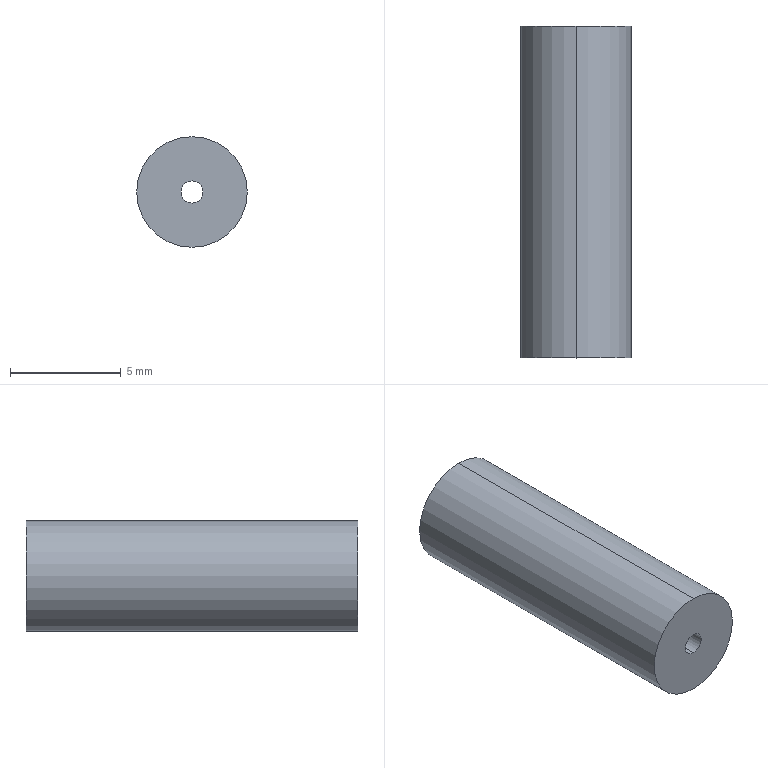Part | SolidWorks | features Extrusion 1, ICE 1 | 1 solid | 9 faces | box 5 x 15 x 5 mm | volume 201.062 mm3 | cylinder 6 | plane 3 | commonest cylinder face diameters 1 x2 3 x2 5 x2
STEP:
#1=CARTESIAN_POINT('',(0.,2.,0.5));
#2=VERTEX_POINT('',#1);
#3=CARTESIAN_POINT('',(0.,2.,-0.5));
#4=VERTEX_POINT('',#3);
#5=CARTESIAN_POINT('',(0.,2.,0.));
#6=DIRECTION('',(0.,-1.,0.));
#7=DIRECTION('',(0.,0.,-1.));
#8=AXIS2_PLACEMENT_3D('',#5,#6,#7);
#9=CIRCLE('',#8,0.5);
#10=EDGE_CURVE('',#2,#4,#9,.T.);
#11=ORIENTED_EDGE('',*,*,#10,.F.);
#12=CARTESIAN_POINT('',(0.,0.,0.5));
#13=VERTEX_POINT('',#12);
#14=CARTESIAN_POINT('',(0.,2.,0.5));
#15=DIRECTION('',(0.,-1.,0.));
#16=VECTOR('',#15,1000.);
#17=LINE('',#14,#16);
#18=EDGE_CURVE('',#2,#13,#17,.T.);
#19=ORIENTED_EDGE('',*,*,#18,.T.);
#20=CARTESIAN_POINT('',(0.,0.,-0.5));
#21=VERTEX_POINT('',#20);
#22=CARTESIAN_POINT('',(0.,0.,0.));
#23=DIRECTION('',(0.,-1.,0.));
#24=DIRECTION('',(0.,0.,-1.));
#25=AXIS2_PLACEMENT_3D('',#22,#23,#24);
#26=CIRCLE('',#25,0.5);
#27=EDGE_CURVE('',#13,#21,#26,.T.);
#28=ORIENTED_EDGE('',*,*,#27,.T.);
#29=CARTESIAN_POINT('',(0.,2.,-0.5));
#30=DIRECTION('',(0.,-1.,0.));
#31=VECTOR('',#30,1000.);
#32=LINE('',#29,#31);
#33=EDGE_CURVE('',#4,#21,#32,.T.);
#34=ORIENTED_EDGE('',*,*,#33,.F.);
#35=EDGE_LOOP('',(#11,#19,#28,#34));
#36=FACE_OUTER_BOUND('',#35,.T.);
#37=CARTESIAN_POINT('',(0.,2.,0.));
#38=DIRECTION('',(0.,-1.,0.));
#39=DIRECTION('',(0.,0.,-1.));
#40=AXIS2_PLACEMENT_3D('',#37,#38,#39);
#41=CYLINDRICAL_SURFACE('',#40,0.5);
#42=ADVANCED_FACE('',(#36),#41,.F.);
#43=CARTESIAN_POINT('',(0.,15.,2.5));
#44=VERTEX_POINT('',#43);
#45=CARTESIAN_POINT('',(0.,15.,-2.5));
#46=VERTEX_POINT('',#45);
#47=CARTESIAN_POINT('',(0.,15.,0.));
#48=DIRECTION('',(0.,1.,0.));
#49=DIRECTION('',(0.,0.,1.));
#50=AXIS2_PLACEMENT_3D('',#47,#48,#49);
#51=CIRCLE('',#50,2.5);
#52=EDGE_CURVE('',#44,#46,#51,.T.);
#53=ORIENTED_EDGE('',*,*,#52,.F.);
#54=CARTESIAN_POINT('',(0.,0.,2.5));
#55=VERTEX_POINT('',#54);
#56=CARTESIAN_POINT('',(0.,15.,2.5));
#57=DIRECTION('',(0.,-1.,0.));
#58=VECTOR('',#57,1000.);
#59=LINE('',#56,#58);
#60=EDGE_CURVE('',#44,#55,#59,.T.);
#61=ORIENTED_EDGE('',*,*,#60,.T.);
#62=CARTESIAN_POINT('',(0.,0.,-2.5));
#63=VERTEX_POINT('',#62);
#64=CARTESIAN_POINT('',(0.,0.,0.));
#65=DIRECTION('',(0.,1.,0.));
#66=DIRECTION('',(0.,0.,1.));
#67=AXIS2_PLACEMENT_3D('',#64,#65,#66);
#68=CIRCLE('',#67,2.5);
#69=EDGE_CURVE('',#55,#63,#68,.T.);
#70=ORIENTED_EDGE('',*,*,#69,.T.);
#71=CARTESIAN_POINT('',(0.,15.,-2.5));
#72=DIRECTION('',(0.,-1.,0.));
#73=VECTOR('',#72,1000.);
#74=LINE('',#71,#73);
#75=EDGE_CURVE('',#46,#63,#74,.T.);
#76=ORIENTED_EDGE('',*,*,#75,.F.);
#77=EDGE_LOOP('',(#53,#61,#70,#76));
#78=FACE_OUTER_BOUND('',#77,.T.);
#79=CARTESIAN_POINT('',(0.,15.,0.));
#80=DIRECTION('',(0.,-1.,0.));
#81=DIRECTION('',(0.,0.,-1.));
#82=AXIS2_PLACEMENT_3D('',#79,#80,#81);
#83=CYLINDRICAL_SURFACE('',#82,2.5);
#84=ADVANCED_FACE('',(#78),#83,.T.);
#85=CARTESIAN_POINT('',(0.,15.,-1.5));
#86=VERTEX_POINT('',#85);
#87=CARTESIAN_POINT('',(0.,15.,1.5));
#88=VERTEX_POINT('',#87);
#89=CARTESIAN_POINT('',(0.,15.,0.));
#90=DIRECTION('',(0.,1.,0.));
#91=DIRECTION('',(0.,0.,1.));
#92=AXIS2_PLACEMENT_3D('',#89,#90,#91);
#93=CIRCLE('',#92,1.5);
#94=EDGE_CURVE('',#86,#88,#93,.T.);
#95=ORIENTED_EDGE('',*,*,#94,.T.);
#96=CARTESIAN_POINT('',(0.,2.,1.5));
#97=VERTEX_POINT('',#96);
#98=CARTESIAN_POINT('',(0.,15.,1.5));
#99=DIRECTION('',(0.,-1.,0.));
#100=VECTOR('',#99,1000.);
#101=LINE('',#98,#100);
#102=EDGE_CURVE('',#88,#97,#101,.T.);
#103=ORIENTED_EDGE('',*,*,#102,.T.);
#104=CARTESIAN_POINT('',(0.,2.,-1.5));
#105=VERTEX_POINT('',#104);
#106=CARTESIAN_POINT('',(0.,2.,0.));
#107=DIRECTION('',(0.,-1.,0.));
#108=DIRECTION('',(0.,0.,-1.));
#109=AXIS2_PLACEMENT_3D('',#106,#107,#108);
#110=CIRCLE('',#109,1.5);
#111=EDGE_CURVE('',#97,#105,#110,.T.);
#112=ORIENTED_EDGE('',*,*,#111,.T.);
#113=CARTESIAN_POINT('',(0.,15.,-1.5));
#114=DIRECTION('',(0.,-1.,0.));
#115=VECTOR('',#114,1000.);
#116=LINE('',#113,#115);
#117=EDGE_CURVE('',#86,#105,#116,.T.);
#118=ORIENTED_EDGE('',*,*,#117,.F.);
#119=EDGE_LOOP('',(#95,#103,#112,#118));
#120=FACE_OUTER_BOUND('',#119,.T.);
#121=CARTESIAN_POINT('',(0.,15.,0.));
#122=DIRECTION('',(0.,-1.,0.));
#123=DIRECTION('',(0.,0.,-1.));
#124=AXIS2_PLACEMENT_3D('',#121,#122,#123);
#125=CYLINDRICAL_SURFACE('',#124,1.5);
#126=ADVANCED_FACE('',(#120),#125,.F.);
#127=ORIENTED_EDGE('',*,*,#102,.F.);
#128=CARTESIAN_POINT('',(0.,15.,0.));
#129=DIRECTION('',(0.,1.,0.));
#130=DIRECTION('',(0.,0.,1.));
#131=AXIS2_PLACEMENT_3D('',#128,#129,#130);
#132=CIRCLE('',#131,1.5);
#133=EDGE_CURVE('',#88,#86,#132,.T.);
#134=ORIENTED_EDGE('',*,*,#133,.T.);
#135=ORIENTED_EDGE('',*,*,#117,.T.);
#136=CARTESIAN_POINT('',(0.,2.,0.));
#137=DIRECTION('',(0.,-1.,0.));
#138=DIRECTION('',(0.,0.,-1.));
#139=AXIS2_PLACEMENT_3D('',#136,#137,#138);
#140=CIRCLE('',#139,1.5);
#141=EDGE_CURVE('',#105,#97,#140,.T.);
#142=ORIENTED_EDGE('',*,*,#141,.T.);
#143=EDGE_LOOP('',(#127,#134,#135,#142));
#144=FACE_OUTER_BOUND('',#143,.T.);
#145=CARTESIAN_POINT('',(0.,15.,0.));
#146=DIRECTION('',(0.,-1.,0.));
#147=DIRECTION('',(0.,0.,-1.));
#148=AXIS2_PLACEMENT_3D('',#145,#146,#147);
#149=CYLINDRICAL_SURFACE('',#148,1.5);
#150=ADVANCED_FACE('',(#144),#149,.F.);
#151=CARTESIAN_POINT('',(0.,15.,0.));
#152=DIRECTION('',(0.,1.,0.));
#153=DIRECTION('',(0.,0.,1.));
#154=AXIS2_PLACEMENT_3D('',#151,#152,#153);
#155=CIRCLE('',#154,2.5);
#156=EDGE_CURVE('',#46,#44,#155,.T.);
#157=ORIENTED_EDGE('',*,*,#156,.T.);
#158=ORIENTED_EDGE('',*,*,#52,.T.);
#159=EDGE_LOOP('',(#157,#158));
#160=FACE_OUTER_BOUND('',#159,.T.);
#161=ORIENTED_EDGE('',*,*,#94,.F.);
#162=ORIENTED_EDGE('',*,*,#133,.F.);
#163=EDGE_LOOP('',(#161,#162));
#164=FACE_BOUND('',#163,.T.);
#165=CARTESIAN_POINT('',(0.,15.,0.));
#166=DIRECTION('',(0.,1.,0.));
#167=DIRECTION('',(0.,0.,1.));
#168=AXIS2_PLACEMENT_3D('',#165,#166,#167);
#169=PLANE('',#168);
#170=ADVANCED_FACE('',(#160,#164),#169,.T.);
#171=CARTESIAN_POINT('',(0.,0.,0.));
#172=DIRECTION('',(0.,1.,0.));
#173=DIRECTION('',(0.,0.,1.));
#174=AXIS2_PLACEMENT_3D('',#171,#172,#173);
#175=CIRCLE('',#174,2.5);
#176=EDGE_CURVE('',#63,#55,#175,.T.);
#177=ORIENTED_EDGE('',*,*,#176,.F.);
#178=ORIENTED_EDGE('',*,*,#69,.F.);
#179=EDGE_LOOP('',(#177,#178));
#180=FACE_OUTER_BOUND('',#179,.T.);
#181=CARTESIAN_POINT('',(0.,0.,0.));
#182=DIRECTION('',(0.,-1.,0.));
#183=DIRECTION('',(0.,0.,-1.));
#184=AXIS2_PLACEMENT_3D('',#181,#182,#183);
#185=CIRCLE('',#184,0.5);
#186=EDGE_CURVE('',#21,#13,#185,.T.);
#187=ORIENTED_EDGE('',*,*,#186,.F.);
#188=ORIENTED_EDGE('',*,*,#27,.F.);
#189=EDGE_LOOP('',(#187,#188));
#190=FACE_BOUND('',#189,.T.);
#191=CARTESIAN_POINT('',(0.,0.,0.));
#192=DIRECTION('',(0.,1.,0.));
#193=DIRECTION('',(0.,0.,1.));
#194=AXIS2_PLACEMENT_3D('',#191,#192,#193);
#195=PLANE('',#194);
#196=ADVANCED_FACE('',(#180,#190),#195,.F.);
#197=ORIENTED_EDGE('',*,*,#60,.F.);
#198=ORIENTED_EDGE('',*,*,#156,.F.);
#199=ORIENTED_EDGE('',*,*,#75,.T.);
#200=ORIENTED_EDGE('',*,*,#176,.T.);
#201=EDGE_LOOP('',(#197,#198,#199,#200));
#202=FACE_OUTER_BOUND('',#201,.T.);
#203=CARTESIAN_POINT('',(0.,15.,0.));
#204=DIRECTION('',(0.,-1.,0.));
#205=DIRECTION('',(0.,0.,-1.));
#206=AXIS2_PLACEMENT_3D('',#203,#204,#205);
#207=CYLINDRICAL_SURFACE('',#206,2.5);
#208=ADVANCED_FACE('',(#202),#207,.T.);
#209=CARTESIAN_POINT('',(0.,2.,0.));
#210=DIRECTION('',(0.,-1.,0.));
#211=DIRECTION('',(0.,0.,-1.));
#212=AXIS2_PLACEMENT_3D('',#209,#210,#211);
#213=CIRCLE('',#212,0.5);
#214=EDGE_CURVE('',#4,#2,#213,.T.);
#215=ORIENTED_EDGE('',*,*,#214,.T.);
#216=ORIENTED_EDGE('',*,*,#10,.T.);
#217=EDGE_LOOP('',(#215,#216));
#218=FACE_BOUND('',#217,.T.);
#219=ORIENTED_EDGE('',*,*,#141,.F.);
#220=ORIENTED_EDGE('',*,*,#111,.F.);
#221=EDGE_LOOP('',(#219,#220));
#222=FACE_OUTER_BOUND('',#221,.T.);
#223=CARTESIAN_POINT('',(0.,2.,0.));
#224=DIRECTION('',(0.,-1.,0.));
#225=DIRECTION('',(0.,0.,-1.));
#226=AXIS2_PLACEMENT_3D('',#223,#224,#225);
#227=PLANE('',#226);
#228=ADVANCED_FACE('',(#218,#222),#227,.F.);
#229=ORIENTED_EDGE('',*,*,#18,.F.);
#230=ORIENTED_EDGE('',*,*,#214,.F.);
#231=ORIENTED_EDGE('',*,*,#33,.T.);
#232=ORIENTED_EDGE('',*,*,#186,.T.);
#233=EDGE_LOOP('',(#229,#230,#231,#232));
#234=FACE_OUTER_BOUND('',#233,.T.);
#235=CARTESIAN_POINT('',(0.,2.,0.));
#236=DIRECTION('',(0.,-1.,0.));
#237=DIRECTION('',(0.,0.,-1.));
#238=AXIS2_PLACEMENT_3D('',#235,#236,#237);
#239=CYLINDRICAL_SURFACE('',#238,0.5);
#240=ADVANCED_FACE('',(#234),#239,.F.);
#241=CLOSED_SHELL('',(#42,#84,#126,#150,#170,#196,#208,#228,#240));
#242=MANIFOLD_SOLID_BREP('',#241);
#243=CARTESIAN_POINT('',(0.,0.,0.));
#244=DIRECTION('',(0.,0.,1.));
#245=DIRECTION('',(1.,0.,0.));
#246=AXIS2_PLACEMENT_3D('',#243,#244,#245);
#247=(LENGTH_UNIT()NAMED_UNIT(*)SI_UNIT(.MILLI.,.METRE.));
#248=UNCERTAINTY_MEASURE_WITH_UNIT(LENGTH_MEASURE(0.00001),#247,'','');
#249=(NAMED_UNIT(*)PLANE_ANGLE_UNIT()SI_UNIT($,.RADIAN.));
#250=(NAMED_UNIT(*)SI_UNIT($,.STERADIAN.)SOLID_ANGLE_UNIT());
#251=(GEOMETRIC_REPRESENTATION_CONTEXT(3)GLOBAL_UNCERTAINTY_ASSIGNED_CONTEXT((#248))GLOBAL_UNIT_ASSIGNED_CONTEXT((#247,#249,#250))REPRESENTATION_CONTEXT('',''));
#252=ADVANCED_BREP_SHAPE_REPRESENTATION('',(#242,#246),#251);